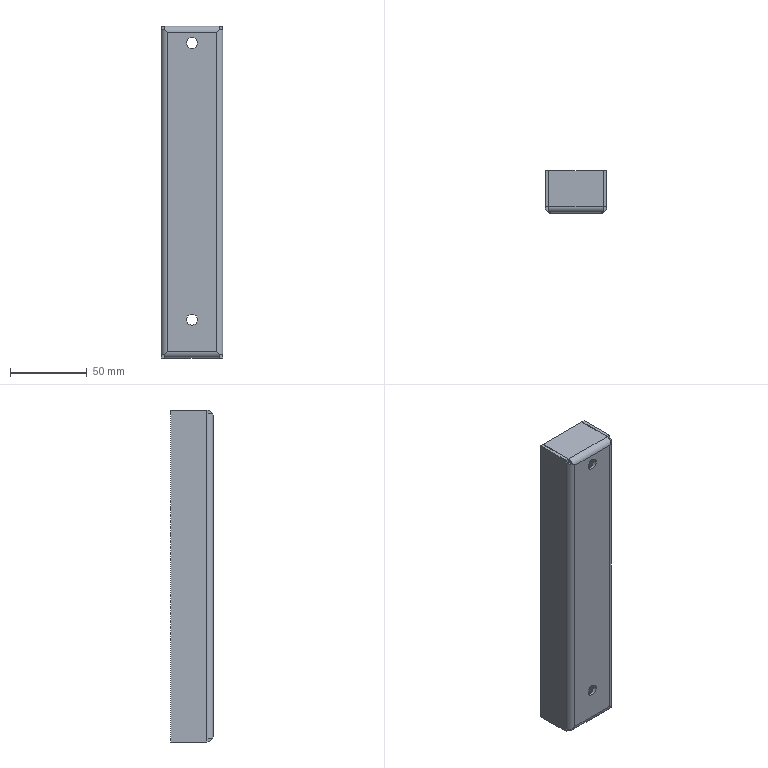Part | NX | features solid 2 | 1 solid | 50 faces | box 40 x 27.5 x 216 mm | volume 41429 mm3 | plane 38 | cylinder 12 | commonest cylinder face diameters 4 x4 7.2 x4 8 x4
STEP:
#1=CARTESIAN_POINT('',(997.,-673.5,1241.));
#2=VERTEX_POINT('',#1);
#3=CARTESIAN_POINT('',(997.,-650.,1241.));
#4=VERTEX_POINT('',#3);
#5=CARTESIAN_POINT('',(997.,-677.5,1241.));
#6=DIRECTION('',(0.,1.,0.));
#7=VECTOR('',#6,1000.);
#8=LINE('',#5,#7);
#9=EDGE_CURVE('',#2,#4,#8,.T.);
#10=ORIENTED_EDGE('',*,*,#9,.F.);
#11=CARTESIAN_POINT('',(997.,-673.5,1238.8));
#12=VERTEX_POINT('',#11);
#13=CARTESIAN_POINT('',(997.,-673.5,1025.));
#14=DIRECTION('',(0.,0.,1.));
#15=VECTOR('',#14,1000.);
#16=LINE('',#13,#15);
#17=EDGE_CURVE('',#12,#2,#16,.T.);
#18=ORIENTED_EDGE('',*,*,#17,.F.);
#19=CARTESIAN_POINT('',(997.,-673.5,1027.2));
#20=VERTEX_POINT('',#19);
#21=CARTESIAN_POINT('',(997.,-673.5,1025.));
#22=DIRECTION('',(0.,0.,1.));
#23=VECTOR('',#22,1000.);
#24=LINE('',#21,#23);
#25=EDGE_CURVE('',#20,#12,#24,.T.);
#26=ORIENTED_EDGE('',*,*,#25,.F.);
#27=CARTESIAN_POINT('',(997.,-673.5,1025.));
#28=VERTEX_POINT('',#27);
#29=CARTESIAN_POINT('',(997.,-673.5,1025.));
#30=DIRECTION('',(0.,0.,1.));
#31=VECTOR('',#30,1000.);
#32=LINE('',#29,#31);
#33=EDGE_CURVE('',#28,#20,#32,.T.);
#34=ORIENTED_EDGE('',*,*,#33,.F.);
#35=CARTESIAN_POINT('',(997.,-650.,1025.));
#36=VERTEX_POINT('',#35);
#37=CARTESIAN_POINT('',(997.,-677.5,1025.));
#38=DIRECTION('',(0.,1.,0.));
#39=VECTOR('',#38,1000.);
#40=LINE('',#37,#39);
#41=EDGE_CURVE('',#28,#36,#40,.T.);
#42=ORIENTED_EDGE('',*,*,#41,.T.);
#43=CARTESIAN_POINT('',(997.,-650.,1025.));
#44=DIRECTION('',(0.,0.,1.));
#45=VECTOR('',#44,1000.);
#46=LINE('',#43,#45);
#47=EDGE_CURVE('',#36,#4,#46,.T.);
#48=ORIENTED_EDGE('',*,*,#47,.T.);
#49=EDGE_LOOP('',(#10,#18,#26,#34,#42,#48));
#50=FACE_BOUND('',#49,.T.);
#51=CARTESIAN_POINT('',(997.,-677.5,1025.));
#52=DIRECTION('',(1.,0.,0.));
#53=DIRECTION('',(0.,0.,-1.));
#54=AXIS2_PLACEMENT_3D('',#51,#52,#53);
#55=PLANE('',#54);
#56=ADVANCED_FACE('',(#50),#55,.T.);
#57=CARTESIAN_POINT('',(995.,-673.5,1241.));
#58=VERTEX_POINT('',#57);
#59=CARTESIAN_POINT('',(995.,-650.,1241.));
#60=VERTEX_POINT('',#59);
#61=CARTESIAN_POINT('',(995.,-677.5,1241.));
#62=DIRECTION('',(0.,1.,0.));
#63=VECTOR('',#62,1000.);
#64=LINE('',#61,#63);
#65=EDGE_CURVE('',#58,#60,#64,.T.);
#66=ORIENTED_EDGE('',*,*,#65,.T.);
#67=CARTESIAN_POINT('',(995.,-650.,1025.));
#68=VERTEX_POINT('',#67);
#69=CARTESIAN_POINT('',(995.,-650.,1025.));
#70=DIRECTION('',(0.,0.,1.));
#71=VECTOR('',#70,1000.);
#72=LINE('',#69,#71);
#73=EDGE_CURVE('',#68,#60,#72,.T.);
#74=ORIENTED_EDGE('',*,*,#73,.F.);
#75=CARTESIAN_POINT('',(995.,-673.5,1025.));
#76=VERTEX_POINT('',#75);
#77=CARTESIAN_POINT('',(995.,-677.5,1025.));
#78=DIRECTION('',(0.,1.,0.));
#79=VECTOR('',#78,1000.);
#80=LINE('',#77,#79);
#81=EDGE_CURVE('',#76,#68,#80,.T.);
#82=ORIENTED_EDGE('',*,*,#81,.F.);
#83=CARTESIAN_POINT('',(995.,-673.5,1027.2));
#84=VERTEX_POINT('',#83);
#85=CARTESIAN_POINT('',(995.,-673.5,1025.));
#86=DIRECTION('',(0.,0.,1.));
#87=VECTOR('',#86,1000.);
#88=LINE('',#85,#87);
#89=EDGE_CURVE('',#76,#84,#88,.T.);
#90=ORIENTED_EDGE('',*,*,#89,.T.);
#91=CARTESIAN_POINT('',(995.,-673.5,1238.8));
#92=VERTEX_POINT('',#91);
#93=CARTESIAN_POINT('',(995.,-673.5,1025.));
#94=DIRECTION('',(0.,0.,1.));
#95=VECTOR('',#94,1000.);
#96=LINE('',#93,#95);
#97=EDGE_CURVE('',#84,#92,#96,.T.);
#98=ORIENTED_EDGE('',*,*,#97,.T.);
#99=CARTESIAN_POINT('',(995.,-673.5,1025.));
#100=DIRECTION('',(0.,0.,1.));
#101=VECTOR('',#100,1000.);
#102=LINE('',#99,#101);
#103=EDGE_CURVE('',#92,#58,#102,.T.);
#104=ORIENTED_EDGE('',*,*,#103,.T.);
#105=EDGE_LOOP('',(#66,#74,#82,#90,#98,#104));
#106=FACE_BOUND('',#105,.T.);
#107=CARTESIAN_POINT('',(995.,-677.5,1025.));
#108=DIRECTION('',(1.,0.,0.));
#109=DIRECTION('',(0.,0.,-1.));
#110=AXIS2_PLACEMENT_3D('',#107,#108,#109);
#111=PLANE('',#110);
#112=ADVANCED_FACE('',(#106),#111,.F.);
#113=CARTESIAN_POINT('',(1024.5,-673.5,1238.8));
#114=DIRECTION('',(-1.,0.,0.));
#115=VECTOR('',#114,1000.);
#116=LINE('',#113,#115);
#117=EDGE_CURVE('',#12,#92,#116,.T.);
#118=ORIENTED_EDGE('',*,*,#117,.F.);
#119=ORIENTED_EDGE('',*,*,#17,.T.);
#120=CARTESIAN_POINT('',(995.,-673.5,1241.));
#121=DIRECTION('',(1.,0.,0.));
#122=VECTOR('',#121,1000.);
#123=LINE('',#120,#122);
#124=EDGE_CURVE('',#58,#2,#123,.T.);
#125=ORIENTED_EDGE('',*,*,#124,.F.);
#126=ORIENTED_EDGE('',*,*,#103,.F.);
#127=EDGE_LOOP('',(#118,#119,#125,#126));
#128=FACE_BOUND('',#127,.T.);
#129=CARTESIAN_POINT('',(995.,-673.5,1025.));
#130=DIRECTION('',(0.,1.,0.));
#131=DIRECTION('',(1.,0.,0.));
#132=AXIS2_PLACEMENT_3D('',#129,#130,#131);
#133=PLANE('',#132);
#134=ADVANCED_FACE('',(#128),#133,.F.);
#135=CARTESIAN_POINT('',(995.,-673.5,1025.));
#136=DIRECTION('',(1.,0.,0.));
#137=VECTOR('',#136,1000.);
#138=LINE('',#135,#137);
#139=EDGE_CURVE('',#76,#28,#138,.T.);
#140=ORIENTED_EDGE('',*,*,#139,.F.);
#141=ORIENTED_EDGE('',*,*,#81,.T.);
#142=CARTESIAN_POINT('',(995.,-650.,1025.));
#143=DIRECTION('',(-1.,0.,0.));
#144=VECTOR('',#143,1000.);
#145=LINE('',#142,#144);
#146=EDGE_CURVE('',#36,#68,#145,.T.);
#147=ORIENTED_EDGE('',*,*,#146,.F.);
#148=ORIENTED_EDGE('',*,*,#41,.F.);
#149=EDGE_LOOP('',(#140,#141,#147,#148));
#150=FACE_BOUND('',#149,.T.);
#151=CARTESIAN_POINT('',(1035.,-677.5,1025.));
#152=DIRECTION('',(0.,0.,-1.));
#153=DIRECTION('',(-1.,0.,0.));
#154=AXIS2_PLACEMENT_3D('',#151,#152,#153);
#155=PLANE('',#154);
#156=ADVANCED_FACE('',(#150),#155,.T.);
#157=ORIENTED_EDGE('',*,*,#124,.T.);
#158=ORIENTED_EDGE('',*,*,#9,.T.);
#159=CARTESIAN_POINT('',(995.,-650.,1241.));
#160=DIRECTION('',(-1.,0.,0.));
#161=VECTOR('',#160,1000.);
#162=LINE('',#159,#161);
#163=EDGE_CURVE('',#4,#60,#162,.T.);
#164=ORIENTED_EDGE('',*,*,#163,.T.);
#165=ORIENTED_EDGE('',*,*,#65,.F.);
#166=EDGE_LOOP('',(#157,#158,#164,#165));
#167=FACE_BOUND('',#166,.T.);
#168=CARTESIAN_POINT('',(1031.,-673.5,1241.));
#169=DIRECTION('',(0.,0.,-1.));
#170=DIRECTION('',(-1.,0.,0.));
#171=AXIS2_PLACEMENT_3D('',#168,#169,#170);
#172=PLANE('',#171);
#173=ADVANCED_FACE('',(#167),#172,.F.);
#174=ORIENTED_EDGE('',*,*,#163,.F.);
#175=ORIENTED_EDGE('',*,*,#47,.F.);
#176=ORIENTED_EDGE('',*,*,#146,.T.);
#177=ORIENTED_EDGE('',*,*,#73,.T.);
#178=EDGE_LOOP('',(#174,#175,#176,#177));
#179=FACE_BOUND('',#178,.T.);
#180=CARTESIAN_POINT('',(995.,-650.,1025.));
#181=DIRECTION('',(0.,1.,0.));
#182=DIRECTION('',(1.,0.,0.));
#183=AXIS2_PLACEMENT_3D('',#180,#181,#182);
#184=PLANE('',#183);
#185=ADVANCED_FACE('',(#179),#184,.T.);
#186=ORIENTED_EDGE('',*,*,#33,.T.);
#187=CARTESIAN_POINT('',(1024.5,-673.5,1027.2));
#188=DIRECTION('',(-1.,0.,0.));
#189=VECTOR('',#188,1000.);
#190=LINE('',#187,#189);
#191=EDGE_CURVE('',#20,#84,#190,.T.);
#192=ORIENTED_EDGE('',*,*,#191,.T.);
#193=ORIENTED_EDGE('',*,*,#89,.F.);
#194=ORIENTED_EDGE('',*,*,#139,.T.);
#195=EDGE_LOOP('',(#186,#192,#193,#194));
#196=FACE_BOUND('',#195,.T.);
#197=CARTESIAN_POINT('',(995.,-673.5,1025.));
#198=DIRECTION('',(0.,1.,0.));
#199=DIRECTION('',(1.,0.,0.));
#200=AXIS2_PLACEMENT_3D('',#197,#198,#199);
#201=PLANE('',#200);
#202=ADVANCED_FACE('',(#196),#201,.F.);
#203=CARTESIAN_POINT('',(997.,-676.964,1238.8));
#204=VERTEX_POINT('',#203);
#205=CARTESIAN_POINT('',(999.,-673.5,1238.8));
#206=DIRECTION('',(0.,0.,-1.));
#207=DIRECTION('',(0.,1.,0.));
#208=AXIS2_PLACEMENT_3D('',#205,#206,#207);
#209=CIRCLE('',#208,4.);
#210=EDGE_CURVE('',#204,#92,#209,.T.);
#211=ORIENTED_EDGE('',*,*,#210,.F.);
#212=CARTESIAN_POINT('',(997.,322.5,1238.8));
#213=DIRECTION('',(0.,1.,0.));
#214=VECTOR('',#213,1000.);
#215=LINE('',#212,#214);
#216=EDGE_CURVE('',#204,#12,#215,.T.);
#217=ORIENTED_EDGE('',*,*,#216,.T.);
#218=ORIENTED_EDGE('',*,*,#117,.T.);
#219=EDGE_LOOP('',(#211,#217,#218));
#220=FACE_BOUND('',#219,.T.);
#221=CARTESIAN_POINT('',(997.,-1677.5,1238.8));
#222=DIRECTION('',(0.,0.,-1.));
#223=DIRECTION('',(-1.,0.,0.));
#224=AXIS2_PLACEMENT_3D('',#221,#222,#223);
#225=PLANE('',#224);
#226=ADVANCED_FACE('',(#220),#225,.F.);
#227=CARTESIAN_POINT('',(999.,-677.5,1237.));
#228=VERTEX_POINT('',#227);
#229=CARTESIAN_POINT('',(999.,-677.5,1237.));
#230=CARTESIAN_POINT('',(998.294,-677.5,1237.636));
#231=CARTESIAN_POINT('',(997.612,-677.317,1238.25));
#232=CARTESIAN_POINT('',(997.,-676.964,1238.8));
#233=(BOUNDED_CURVE()B_SPLINE_CURVE(3,(#229,#230,#231,#232),.UNSPECIFIED.,.F.,.F.)B_SPLINE_CURVE_WITH_KNOTS((4,4),(4.712,5.236),.PIECEWISE_BEZIER_KNOTS.)CURVE()GEOMETRIC_REPRESENTATION_ITEM()RATIONAL_B_SPLINE_CURVE((1.,0.9773,0.9773,1.))REPRESENTATION_ITEM(''));
#234=EDGE_CURVE('',#228,#204,#233,.T.);
#235=ORIENTED_EDGE('',*,*,#234,.F.);
#236=CARTESIAN_POINT('',(999.,-675.5,1237.));
#237=VERTEX_POINT('',#236);
#238=CARTESIAN_POINT('',(999.,-675.5,1237.));
#239=DIRECTION('',(0.,-1.,0.));
#240=VECTOR('',#239,1000.);
#241=LINE('',#238,#240);
#242=EDGE_CURVE('',#237,#228,#241,.T.);
#243=ORIENTED_EDGE('',*,*,#242,.F.);
#244=CARTESIAN_POINT('',(999.,-675.5,1237.));
#245=CARTESIAN_POINT('',(997.828,-675.5,1238.054));
#246=CARTESIAN_POINT('',(997.,-674.672,1238.8));
#247=CARTESIAN_POINT('',(997.,-673.5,1238.8));
#248=(BOUNDED_CURVE()B_SPLINE_CURVE(3,(#244,#245,#246,#247),.UNSPECIFIED.,.F.,.F.)B_SPLINE_CURVE_WITH_KNOTS((4,4),(4.712,6.283),.PIECEWISE_BEZIER_KNOTS.)CURVE()GEOMETRIC_REPRESENTATION_ITEM()RATIONAL_B_SPLINE_CURVE((1.,0.8047,0.8047,1.))REPRESENTATION_ITEM(''));
#249=EDGE_CURVE('',#237,#12,#248,.T.);
#250=ORIENTED_EDGE('',*,*,#249,.T.);
#251=ORIENTED_EDGE('',*,*,#216,.F.);
#252=EDGE_LOOP('',(#235,#243,#250,#251));
#253=FACE_BOUND('',#252,.T.);
#254=CARTESIAN_POINT('',(1742.294,-1677.5,568.035));
#255=DIRECTION('',(-0.669,0.,-0.7433));
#256=DIRECTION('',(-0.7433,0.,0.669));
#257=AXIS2_PLACEMENT_3D('',#254,#255,#256);
#258=PLANE('',#257);
#259=ADVANCED_FACE('',(#253),#258,.F.);
#260=CARTESIAN_POINT('',(997.,-676.964,1027.2));
#261=VERTEX_POINT('',#260);
#262=CARTESIAN_POINT('',(997.,322.5,1027.2));
#263=DIRECTION('',(0.,1.,0.));
#264=VECTOR('',#263,1000.);
#265=LINE('',#262,#264);
#266=EDGE_CURVE('',#261,#20,#265,.T.);
#267=ORIENTED_EDGE('',*,*,#266,.F.);
#268=CARTESIAN_POINT('',(999.,-673.5,1027.2));
#269=DIRECTION('',(0.,0.,-1.));
#270=DIRECTION('',(0.,1.,0.));
#271=AXIS2_PLACEMENT_3D('',#268,#269,#270);
#272=CIRCLE('',#271,4.);
#273=EDGE_CURVE('',#261,#84,#272,.T.);
#274=ORIENTED_EDGE('',*,*,#273,.T.);
#275=ORIENTED_EDGE('',*,*,#191,.F.);
#276=EDGE_LOOP('',(#267,#274,#275));
#277=FACE_BOUND('',#276,.T.);
#278=CARTESIAN_POINT('',(997.,-1677.5,1027.2));
#279=DIRECTION('',(0.,0.,-1.));
#280=DIRECTION('',(-1.,0.,0.));
#281=AXIS2_PLACEMENT_3D('',#278,#279,#280);
#282=PLANE('',#281);
#283=ADVANCED_FACE('',(#277),#282,.T.);
#284=CARTESIAN_POINT('',(999.,-675.5,1029.));
#285=VERTEX_POINT('',#284);
#286=CARTESIAN_POINT('',(999.,-677.5,1029.));
#287=VERTEX_POINT('',#286);
#288=CARTESIAN_POINT('',(999.,-675.5,1029.));
#289=DIRECTION('',(0.,-1.,0.));
#290=VECTOR('',#289,1000.);
#291=LINE('',#288,#290);
#292=EDGE_CURVE('',#285,#287,#291,.T.);
#293=ORIENTED_EDGE('',*,*,#292,.T.);
#294=CARTESIAN_POINT('',(999.,-677.5,1029.));
#295=CARTESIAN_POINT('',(998.294,-677.5,1028.364));
#296=CARTESIAN_POINT('',(997.612,-677.317,1027.75));
#297=CARTESIAN_POINT('',(997.,-676.964,1027.2));
#298=(BOUNDED_CURVE()B_SPLINE_CURVE(3,(#294,#295,#296,#297),.UNSPECIFIED.,.F.,.F.)B_SPLINE_CURVE_WITH_KNOTS((4,4),(1.571,2.094),.PIECEWISE_BEZIER_KNOTS.)CURVE()GEOMETRIC_REPRESENTATION_ITEM()RATIONAL_B_SPLINE_CURVE((1.,0.9773,0.9773,1.))REPRESENTATION_ITEM(''));
#299=EDGE_CURVE('',#287,#261,#298,.T.);
#300=ORIENTED_EDGE('',*,*,#299,.T.);
#301=ORIENTED_EDGE('',*,*,#266,.T.);
#302=CARTESIAN_POINT('',(999.,-675.5,1029.));
#303=CARTESIAN_POINT('',(997.828,-675.5,1027.946));
#304=CARTESIAN_POINT('',(997.,-674.672,1027.2));
#305=CARTESIAN_POINT('',(997.,-673.5,1027.2));
#306=(BOUNDED_CURVE()B_SPLINE_CURVE(3,(#302,#303,#304,#305),.UNSPECIFIED.,.F.,.F.)B_SPLINE_CURVE_WITH_KNOTS((4,4),(1.571,3.142),.PIECEWISE_BEZIER_KNOTS.)CURVE()GEOMETRIC_REPRESENTATION_ITEM()RATIONAL_B_SPLINE_CURVE((1.,0.8047,0.8047,1.))REPRESENTATION_ITEM(''));
#307=EDGE_CURVE('',#285,#20,#306,.T.);
#308=ORIENTED_EDGE('',*,*,#307,.F.);
#309=EDGE_LOOP('',(#293,#300,#301,#308));
#310=FACE_BOUND('',#309,.T.);
#311=CARTESIAN_POINT('',(1742.294,-1677.5,1697.965));
#312=DIRECTION('',(0.669,0.,-0.7433));
#313=DIRECTION('',(0.,-1.,0.));
#314=AXIS2_PLACEMENT_3D('',#311,#312,#313);
#315=PLANE('',#314);
#316=ADVANCED_FACE('',(#310),#315,.T.);
#317=ORIENTED_EDGE('',*,*,#249,.F.);
#318=CARTESIAN_POINT('',(999.,-675.5,1025.));
#319=DIRECTION('',(0.,0.,1.));
#320=VECTOR('',#319,1000.);
#321=LINE('',#318,#320);
#322=EDGE_CURVE('',#285,#237,#321,.T.);
#323=ORIENTED_EDGE('',*,*,#322,.F.);
#324=ORIENTED_EDGE('',*,*,#307,.T.);
#325=ORIENTED_EDGE('',*,*,#25,.T.);
#326=EDGE_LOOP('',(#317,#323,#324,#325));
#327=FACE_BOUND('',#326,.T.);
#328=CARTESIAN_POINT('',(999.,-673.5,1025.));
#329=DIRECTION('',(0.,0.,1.));
#330=DIRECTION('',(0.,-1.,0.));
#331=AXIS2_PLACEMENT_3D('',#328,#329,#330);
#332=CYLINDRICAL_SURFACE('',#331,2.);
#333=ADVANCED_FACE('',(#327),#332,.F.);
#334=CARTESIAN_POINT('',(999.,-677.5,1025.));
#335=DIRECTION('',(0.,0.,1.));
#336=VECTOR('',#335,1000.);
#337=LINE('',#334,#336);
#338=EDGE_CURVE('',#287,#228,#337,.T.);
#339=ORIENTED_EDGE('',*,*,#338,.T.);
#340=ORIENTED_EDGE('',*,*,#234,.T.);
#341=ORIENTED_EDGE('',*,*,#210,.T.);
#342=ORIENTED_EDGE('',*,*,#97,.F.);
#343=ORIENTED_EDGE('',*,*,#273,.F.);
#344=ORIENTED_EDGE('',*,*,#299,.F.);
#345=EDGE_LOOP('',(#339,#340,#341,#342,#343,#344));
#346=FACE_BOUND('',#345,.T.);
#347=CARTESIAN_POINT('',(999.,-673.5,1025.));
#348=DIRECTION('',(0.,0.,1.));
#349=DIRECTION('',(0.,-1.,0.));
#350=AXIS2_PLACEMENT_3D('',#347,#348,#349);
#351=CYLINDRICAL_SURFACE('',#350,4.);
#352=ADVANCED_FACE('',(#346),#351,.T.);
#353=CARTESIAN_POINT('',(997.2,-650.,1241.));
#354=VERTEX_POINT('',#353);
#355=CARTESIAN_POINT('',(997.2,-673.5,1241.));
#356=VERTEX_POINT('',#355);
#357=CARTESIAN_POINT('',(997.2,-675.778,1241.));
#358=DIRECTION('',(0.,-1.,0.));
#359=VECTOR('',#358,1000.);
#360=LINE('',#357,#359);
#361=EDGE_CURVE('',#354,#356,#360,.T.);
#362=ORIENTED_EDGE('',*,*,#361,.T.);
#363=CARTESIAN_POINT('',(1032.8,-673.5,1241.));
#364=VERTEX_POINT('',#363);
#365=CARTESIAN_POINT('',(999.,-673.5,1241.));
#366=DIRECTION('',(1.,0.,0.));
#367=VECTOR('',#366,1000.);
#368=LINE('',#365,#367);
#369=EDGE_CURVE('',#356,#364,#368,.T.);
#370=ORIENTED_EDGE('',*,*,#369,.T.);
#371=CARTESIAN_POINT('',(1032.8,-650.,1241.));
#372=VERTEX_POINT('',#371);
#373=CARTESIAN_POINT('',(1032.8,-675.778,1241.));
#374=DIRECTION('',(0.,1.,0.));
#375=VECTOR('',#374,1000.);
#376=LINE('',#373,#375);
#377=EDGE_CURVE('',#364,#372,#376,.T.);
#378=ORIENTED_EDGE('',*,*,#377,.T.);
#379=CARTESIAN_POINT('',(1031.,-650.,1241.));
#380=DIRECTION('',(-1.,0.,0.));
#381=VECTOR('',#380,1000.);
#382=LINE('',#379,#381);
#383=EDGE_CURVE('',#372,#354,#382,.T.);
#384=ORIENTED_EDGE('',*,*,#383,.T.);
#385=EDGE_LOOP('',(#362,#370,#378,#384));
#386=FACE_BOUND('',#385,.T.);
#387=CARTESIAN_POINT('',(1024.5,-552.5,1241.));
#388=DIRECTION('',(0.,0.,1.));
#389=DIRECTION('',(1.,0.,0.));
#390=AXIS2_PLACEMENT_3D('',#387,#388,#389);
#391=PLANE('',#390);
#392=ADVANCED_FACE('',(#386),#391,.T.);
#393=CARTESIAN_POINT('',(997.2,-673.5,1239.));
#394=VERTEX_POINT('',#393);
#395=CARTESIAN_POINT('',(1032.8,-673.5,1239.));
#396=VERTEX_POINT('',#395);
#397=CARTESIAN_POINT('',(999.,-673.5,1239.));
#398=DIRECTION('',(1.,0.,0.));
#399=VECTOR('',#398,1000.);
#400=LINE('',#397,#399);
#401=EDGE_CURVE('',#394,#396,#400,.T.);
#402=ORIENTED_EDGE('',*,*,#401,.F.);
#403=CARTESIAN_POINT('',(997.2,-650.,1239.));
#404=VERTEX_POINT('',#403);
#405=CARTESIAN_POINT('',(997.2,-675.778,1239.));
#406=DIRECTION('',(0.,-1.,0.));
#407=VECTOR('',#406,1000.);
#408=LINE('',#405,#407);
#409=EDGE_CURVE('',#404,#394,#408,.T.);
#410=ORIENTED_EDGE('',*,*,#409,.F.);
#411=CARTESIAN_POINT('',(1032.8,-650.,1239.));
#412=VERTEX_POINT('',#411);
#413=CARTESIAN_POINT('',(1031.,-650.,1239.));
#414=DIRECTION('',(-1.,0.,0.));
#415=VECTOR('',#414,1000.);
#416=LINE('',#413,#415);
#417=EDGE_CURVE('',#412,#404,#416,.T.);
#418=ORIENTED_EDGE('',*,*,#417,.F.);
#419=CARTESIAN_POINT('',(1032.8,-675.778,1239.));
#420=DIRECTION('',(0.,1.,0.));
#421=VECTOR('',#420,1000.);
#422=LINE('',#419,#421);
#423=EDGE_CURVE('',#396,#412,#422,.T.);
#424=ORIENTED_EDGE('',*,*,#423,.F.);
#425=EDGE_LOOP('',(#402,#410,#418,#424));
#426=FACE_BOUND('',#425,.T.);
#427=CARTESIAN_POINT('',(1024.5,-552.5,1239.));
#428=DIRECTION('',(0.,0.,1.));
#429=DIRECTION('',(1.,0.,0.));
#430=AXIS2_PLACEMENT_3D('',#427,#428,#429);
#431=PLANE('',#430);
#432=ADVANCED_FACE('',(#426),#431,.F.);
#433=ORIENTED_EDGE('',*,*,#417,.T.);
#434=CARTESIAN_POINT('',(997.2,-650.,1241.));
#435=DIRECTION('',(0.,0.,-1.));
#436=VECTOR('',#435,1000.);
#437=LINE('',#434,#436);
#438=EDGE_CURVE('',#354,#404,#437,.T.);
#439=ORIENTED_EDGE('',*,*,#438,.F.);
#440=ORIENTED_EDGE('',*,*,#383,.F.);
#441=CARTESIAN_POINT('',(1032.8,-650.,1241.));
#442=DIRECTION('',(0.,0.,-1.));
#443=VECTOR('',#442,1000.);
#444=LINE('',#441,#443);
#445=EDGE_CURVE('',#372,#412,#444,.T.);
#446=ORIENTED_EDGE('',*,*,#445,.T.);
#447=EDGE_LOOP('',(#433,#439,#440,#446));
#448=FACE_BOUND('',#447,.T.);
#449=CARTESIAN_POINT('',(1031.,-650.,1241.));
#450=DIRECTION('',(0.,-1.,0.));
#451=DIRECTION('',(0.,0.,-1.));
#452=AXIS2_PLACEMENT_3D('',#449,#450,#451);
#453=PLANE('',#452);
#454=ADVANCED_FACE('',(#448),#453,.F.);
#455=CARTESIAN_POINT('',(997.2,-676.964,1239.));
#456=VERTEX_POINT('',#455);
#457=CARTESIAN_POINT('',(997.2,-673.5,1237.));
#458=DIRECTION('',(1.,0.,0.));
#459=DIRECTION('',(0.,0.,-1.));
#460=AXIS2_PLACEMENT_3D('',#457,#458,#459);
#461=CIRCLE('',#460,4.);
#462=EDGE_CURVE('',#356,#456,#461,.T.);
#463=ORIENTED_EDGE('',*,*,#462,.F.);
#464=ORIENTED_EDGE('',*,*,#361,.F.);
#465=ORIENTED_EDGE('',*,*,#438,.T.);
#466=ORIENTED_EDGE('',*,*,#409,.T.);
#467=CARTESIAN_POINT('',(997.2,322.5,1239.));
#468=DIRECTION('',(0.,1.,0.));
#469=VECTOR('',#468,1000.);
#470=LINE('',#467,#469);
#471=EDGE_CURVE('',#456,#394,#470,.T.);
#472=ORIENTED_EDGE('',*,*,#471,.F.);
#473=EDGE_LOOP('',(#463,#464,#465,#466,#472));
#474=FACE_BOUND('',#473,.T.);
#475=CARTESIAN_POINT('',(997.2,-1677.5,1239.));
#476=DIRECTION('',(-1.,0.,0.));
#477=DIRECTION('',(0.,1.,0.));
#478=AXIS2_PLACEMENT_3D('',#475,#476,#477);
#479=PLANE('',#478);
#480=ADVANCED_FACE('',(#474),#479,.T.);
#481=ORIENTED_EDGE('',*,*,#471,.T.);
#482=CARTESIAN_POINT('',(997.2,-673.5,1239.));
#483=CARTESIAN_POINT('',(997.2,-674.672,1239.));
#484=CARTESIAN_POINT('',(997.946,-675.5,1238.172));
#485=CARTESIAN_POINT('',(999.,-675.5,1237.));
#486=(BOUNDED_CURVE()B_SPLINE_CURVE(3,(#482,#483,#484,#485),.UNSPECIFIED.,.F.,.F.)B_SPLINE_CURVE_WITH_KNOTS((4,4),(0.,1.571),.PIECEWISE_BEZIER_KNOTS.)CURVE()GEOMETRIC_REPRESENTATION_ITEM()RATIONAL_B_SPLINE_CURVE((1.,0.8047,0.8047,1.))REPRESENTATION_ITEM(''));
#487=EDGE_CURVE('',#394,#237,#486,.T.);
#488=ORIENTED_EDGE('',*,*,#487,.T.);
#489=ORIENTED_EDGE('',*,*,#242,.T.);
#490=CARTESIAN_POINT('',(997.2,-676.964,1239.));
#491=CARTESIAN_POINT('',(997.75,-677.317,1238.388));
#492=CARTESIAN_POINT('',(998.364,-677.5,1237.706));
#493=CARTESIAN_POINT('',(999.,-677.5,1237.));
#494=(BOUNDED_CURVE()B_SPLINE_CURVE(3,(#490,#491,#492,#493),.UNSPECIFIED.,.F.,.F.)B_SPLINE_CURVE_WITH_KNOTS((4,4),(1.047,1.571),.PIECEWISE_BEZIER_KNOTS.)CURVE()GEOMETRIC_REPRESENTATION_ITEM()RATIONAL_B_SPLINE_CURVE((1.,0.9773,0.9773,1.))REPRESENTATION_ITEM(''));
#495=EDGE_CURVE('',#456,#228,#494,.T.);
#496=ORIENTED_EDGE('',*,*,#495,.F.);
#497=EDGE_LOOP('',(#481,#488,#489,#496));
#498=FACE_BOUND('',#497,.T.);
#499=CARTESIAN_POINT('',(1667.965,-1677.5,493.706));
#500=DIRECTION('',(-0.7433,0.,-0.669));
#501=DIRECTION('',(-0.669,0.,0.7433));
#502=AXIS2_PLACEMENT_3D('',#499,#500,#501);
#503=PLANE('',#502);
#504=ADVANCED_FACE('',(#498),#503,.T.);
#505=CARTESIAN_POINT('',(1032.8,-676.964,1239.));
#506=VERTEX_POINT('',#505);
#507=CARTESIAN_POINT('',(1032.8,322.5,1239.));
#508=DIRECTION('',(0.,1.,0.));
#509=VECTOR('',#508,1000.);
#510=LINE('',#507,#509);
#511=EDGE_CURVE('',#506,#396,#510,.T.);
#512=ORIENTED_EDGE('',*,*,#511,.T.);
#513=ORIENTED_EDGE('',*,*,#423,.T.);
#514=ORIENTED_EDGE('',*,*,#445,.F.);
#515=ORIENTED_EDGE('',*,*,#377,.F.);
#516=CARTESIAN_POINT('',(1032.8,-673.5,1237.));
#517=DIRECTION('',(1.,0.,0.));
#518=DIRECTION('',(0.,-1.,0.));
#519=AXIS2_PLACEMENT_3D('',#516,#517,#518);
#520=CIRCLE('',#519,4.);
#521=EDGE_CURVE('',#364,#506,#520,.T.);
#522=ORIENTED_EDGE('',*,*,#521,.T.);
#523=EDGE_LOOP('',(#512,#513,#514,#515,#522));
#524=FACE_BOUND('',#523,.T.);
#525=CARTESIAN_POINT('',(1032.8,-1677.5,1239.));
#526=DIRECTION('',(-1.,0.,0.));
#527=DIRECTION('',(0.,1.,0.));
#528=AXIS2_PLACEMENT_3D('',#525,#526,#527);
#529=PLANE('',#528);
#530=ADVANCED_FACE('',(#524),#529,.F.);
#531=ORIENTED_EDGE('',*,*,#511,.F.);
#532=CARTESIAN_POINT('',(1031.,-677.5,1237.));
#533=VERTEX_POINT('',#532);
#534=CARTESIAN_POINT('',(1032.8,-676.964,1239.));
#535=CARTESIAN_POINT('',(1032.25,-677.317,1238.388));
#536=CARTESIAN_POINT('',(1031.636,-677.5,1237.706));
#537=CARTESIAN_POINT('',(1031.,-677.5,1237.));
#538=(BOUNDED_CURVE()B_SPLINE_CURVE(3,(#534,#535,#536,#537),.UNSPECIFIED.,.F.,.F.)B_SPLINE_CURVE_WITH_KNOTS((4,4),(4.189,4.712),.PIECEWISE_BEZIER_KNOTS.)CURVE()GEOMETRIC_REPRESENTATION_ITEM()RATIONAL_B_SPLINE_CURVE((1.,0.9773,0.9773,1.))REPRESENTATION_ITEM(''));
#539=EDGE_CURVE('',#506,#533,#538,.T.);
#540=ORIENTED_EDGE('',*,*,#539,.T.);
#541=CARTESIAN_POINT('',(1031.,-675.5,1237.));
#542=VERTEX_POINT('',#541);
#543=CARTESIAN_POINT('',(1031.,-675.5,1237.));
#544=DIRECTION('',(0.,-1.,0.));
#545=VECTOR('',#544,1000.);
#546=LINE('',#543,#545);
#547=EDGE_CURVE('',#542,#533,#546,.T.);
#548=ORIENTED_EDGE('',*,*,#547,.F.);
#549=CARTESIAN_POINT('',(1032.8,-673.5,1239.));
#550=CARTESIAN_POINT('',(1032.8,-674.672,1239.));
#551=CARTESIAN_POINT('',(1032.054,-675.5,1238.172));
#552=CARTESIAN_POINT('',(1031.,-675.5,1237.));
#553=(BOUNDED_CURVE()B_SPLINE_CURVE(3,(#549,#550,#551,#552),.UNSPECIFIED.,.F.,.F.)B_SPLINE_CURVE_WITH_KNOTS((4,4),(3.142,4.712),.PIECEWISE_BEZIER_KNOTS.)CURVE()GEOMETRIC_REPRESENTATION_ITEM()RATIONAL_B_SPLINE_CURVE((1.,0.8047,0.8047,1.))REPRESENTATION_ITEM(''));
#554=EDGE_CURVE('',#396,#542,#553,.T.);
#555=ORIENTED_EDGE('',*,*,#554,.F.);
#556=EDGE_LOOP('',(#531,#540,#548,#555));
#557=FACE_BOUND('',#556,.T.);
#558=CARTESIAN_POINT('',(362.035,-1677.5,493.706));
#559=DIRECTION('',(-0.7433,0.,0.669));
#560=DIRECTION('',(0.,1.,0.));
#561=AXIS2_PLACEMENT_3D('',#558,#559,#560);
#562=PLANE('',#561);
#563=ADVANCED_FACE('',(#557),#562,.F.);
#564=ORIENTED_EDGE('',*,*,#462,.T.);
#565=ORIENTED_EDGE('',*,*,#495,.T.);
#566=CARTESIAN_POINT('',(1031.,-677.5,1237.));
#567=DIRECTION('',(-1.,0.,0.));
#568=VECTOR('',#567,1000.);
#569=LINE('',#566,#568);
#570=EDGE_CURVE('',#533,#228,#569,.T.);
#571=ORIENTED_EDGE('',*,*,#570,.F.);
#572=ORIENTED_EDGE('',*,*,#539,.F.);
#573=ORIENTED_EDGE('',*,*,#521,.F.);
#574=ORIENTED_EDGE('',*,*,#369,.F.);
#575=EDGE_LOOP('',(#564,#565,#571,#572,#573,#574));
#576=FACE_BOUND('',#575,.T.);
#577=CARTESIAN_POINT('',(1031.,-673.5,1237.));
#578=DIRECTION('',(-1.,0.,0.));
#579=DIRECTION('',(0.,1.,0.));
#580=AXIS2_PLACEMENT_3D('',#577,#578,#579);
#581=CYLINDRICAL_SURFACE('',#580,4.);
#582=ADVANCED_FACE('',(#576),#581,.T.);
#583=ORIENTED_EDGE('',*,*,#487,.F.);
#584=ORIENTED_EDGE('',*,*,#401,.T.);
#585=ORIENTED_EDGE('',*,*,#554,.T.);
#586=CARTESIAN_POINT('',(1031.,-675.5,1237.));
#587=DIRECTION('',(-1.,0.,0.));
#588=VECTOR('',#587,1000.);
#589=LINE('',#586,#588);
#590=EDGE_CURVE('',#542,#237,#589,.T.);
#591=ORIENTED_EDGE('',*,*,#590,.T.);
#592=EDGE_LOOP('',(#583,#584,#585,#591));
#593=FACE_BOUND('',#592,.T.);
#594=CARTESIAN_POINT('',(1031.,-673.5,1237.));
#595=DIRECTION('',(-1.,0.,0.));
#596=DIRECTION('',(0.,1.,0.));
#597=AXIS2_PLACEMENT_3D('',#594,#595,#596);
#598=CYLINDRICAL_SURFACE('',#597,2.);
#599=ADVANCED_FACE('',(#593),#598,.F.);
#600=CARTESIAN_POINT('',(1035.,-650.,1241.));
#601=VERTEX_POINT('',#600);
#602=CARTESIAN_POINT('',(1035.,-673.5,1241.));
#603=VERTEX_POINT('',#602);
#604=CARTESIAN_POINT('',(1035.,-677.5,1241.));
#605=DIRECTION('',(0.,-1.,0.));
#606=VECTOR('',#605,1000.);
#607=LINE('',#604,#606);
#608=EDGE_CURVE('',#601,#603,#607,.T.);
#609=ORIENTED_EDGE('',*,*,#608,.T.);
#610=CARTESIAN_POINT('',(1035.,-673.5,1238.8));
#611=VERTEX_POINT('',#610);
#612=CARTESIAN_POINT('',(1035.,-673.5,1025.));
#613=DIRECTION('',(0.,0.,1.));
#614=VECTOR('',#613,1000.);
#615=LINE('',#612,#614);
#616=EDGE_CURVE('',#611,#603,#615,.T.);
#617=ORIENTED_EDGE('',*,*,#616,.F.);
#618=CARTESIAN_POINT('',(1035.,-673.5,1027.2));
#619=VERTEX_POINT('',#618);
#620=CARTESIAN_POINT('',(1035.,-673.5,1025.));
#621=DIRECTION('',(0.,0.,1.));
#622=VECTOR('',#621,1000.);
#623=LINE('',#620,#622);
#624=EDGE_CURVE('',#619,#611,#623,.T.);
#625=ORIENTED_EDGE('',*,*,#624,.F.);
#626=CARTESIAN_POINT('',(1035.,-673.5,1025.));
#627=VERTEX_POINT('',#626);
#628=CARTESIAN_POINT('',(1035.,-673.5,1025.));
#629=DIRECTION('',(0.,0.,1.));
#630=VECTOR('',#629,1000.);
#631=LINE('',#628,#630);
#632=EDGE_CURVE('',#627,#619,#631,.T.);
#633=ORIENTED_EDGE('',*,*,#632,.F.);
#634=CARTESIAN_POINT('',(1035.,-650.,1025.));
#635=VERTEX_POINT('',#634);
#636=CARTESIAN_POINT('',(1035.,-677.5,1025.));
#637=DIRECTION('',(0.,-1.,0.));
#638=VECTOR('',#637,1000.);
#639=LINE('',#636,#638);
#640=EDGE_CURVE('',#635,#627,#639,.T.);
#641=ORIENTED_EDGE('',*,*,#640,.F.);
#642=CARTESIAN_POINT('',(1035.,-650.,1025.));
#643=DIRECTION('',(0.,0.,1.));
#644=VECTOR('',#643,1000.);
#645=LINE('',#642,#644);
#646=EDGE_CURVE('',#635,#601,#645,.T.);
#647=ORIENTED_EDGE('',*,*,#646,.T.);
#648=EDGE_LOOP('',(#609,#617,#625,#633,#641,#647));
#649=FACE_BOUND('',#648,.T.);
#650=CARTESIAN_POINT('',(1035.,-677.5,1025.));
#651=DIRECTION('',(-1.,0.,0.));
#652=DIRECTION('',(0.,1.,0.));
#653=AXIS2_PLACEMENT_3D('',#650,#651,#652);
#654=PLANE('',#653);
#655=ADVANCED_FACE('',(#649),#654,.F.);
#656=CARTESIAN_POINT('',(1033.,-650.,1241.));
#657=VERTEX_POINT('',#656);
#658=CARTESIAN_POINT('',(1033.,-673.5,1241.));
#659=VERTEX_POINT('',#658);
#660=CARTESIAN_POINT('',(1033.,-677.5,1241.));
#661=DIRECTION('',(0.,-1.,0.));
#662=VECTOR('',#661,1000.);
#663=LINE('',#660,#662);
#664=EDGE_CURVE('',#657,#659,#663,.T.);
#665=ORIENTED_EDGE('',*,*,#664,.F.);
#666=CARTESIAN_POINT('',(1033.,-650.,1025.));
#667=VERTEX_POINT('',#666);
#668=CARTESIAN_POINT('',(1033.,-650.,1025.));
#669=DIRECTION('',(0.,0.,1.));
#670=VECTOR('',#669,1000.);
#671=LINE('',#668,#670);
#672=EDGE_CURVE('',#667,#657,#671,.T.);
#673=ORIENTED_EDGE('',*,*,#672,.F.);
#674=CARTESIAN_POINT('',(1033.,-673.5,1025.));
#675=VERTEX_POINT('',#674);
#676=CARTESIAN_POINT('',(1033.,-677.5,1025.));
#677=DIRECTION('',(0.,-1.,0.));
#678=VECTOR('',#677,1000.);
#679=LINE('',#676,#678);
#680=EDGE_CURVE('',#667,#675,#679,.T.);
#681=ORIENTED_EDGE('',*,*,#680,.T.);
#682=CARTESIAN_POINT('',(1033.,-673.5,1027.2));
#683=VERTEX_POINT('',#682);
#684=CARTESIAN_POINT('',(1033.,-673.5,1025.));
#685=DIRECTION('',(0.,0.,1.));
#686=VECTOR('',#685,1000.);
#687=LINE('',#684,#686);
#688=EDGE_CURVE('',#675,#683,#687,.T.);
#689=ORIENTED_EDGE('',*,*,#688,.T.);
#690=CARTESIAN_POINT('',(1033.,-673.5,1238.8));
#691=VERTEX_POINT('',#690);
#692=CARTESIAN_POINT('',(1033.,-673.5,1025.));
#693=DIRECTION('',(0.,0.,1.));
#694=VECTOR('',#693,1000.);
#695=LINE('',#692,#694);
#696=EDGE_CURVE('',#683,#691,#695,.T.);
#697=ORIENTED_EDGE('',*,*,#696,.T.);
#698=CARTESIAN_POINT('',(1033.,-673.5,1025.));
#699=DIRECTION('',(0.,0.,1.));
#700=VECTOR('',#699,1000.);
#701=LINE('',#698,#700);
#702=EDGE_CURVE('',#691,#659,#701,.T.);
#703=ORIENTED_EDGE('',*,*,#702,.T.);
#704=EDGE_LOOP('',(#665,#673,#681,#689,#697,#703));
#705=FACE_BOUND('',#704,.T.);
#706=CARTESIAN_POINT('',(1033.,-677.5,1025.));
#707=DIRECTION('',(-1.,0.,0.));
#708=DIRECTION('',(0.,1.,0.));
#709=AXIS2_PLACEMENT_3D('',#706,#707,#708);
#710=PLANE('',#709);
#711=ADVANCED_FACE('',(#705),#710,.T.);
#712=ORIENTED_EDGE('',*,*,#632,.T.);
#713=CARTESIAN_POINT('',(1024.5,-673.5,1027.2));
#714=DIRECTION('',(-1.,0.,0.));
#715=VECTOR('',#714,1000.);
#716=LINE('',#713,#715);
#717=EDGE_CURVE('',#619,#683,#716,.T.);
#718=ORIENTED_EDGE('',*,*,#717,.T.);
#719=ORIENTED_EDGE('',*,*,#688,.F.);
#720=CARTESIAN_POINT('',(1035.,-673.5,1025.));
#721=DIRECTION('',(-1.,0.,0.));
#722=VECTOR('',#721,1000.);
#723=LINE('',#720,#722);
#724=EDGE_CURVE('',#627,#675,#723,.T.);
#725=ORIENTED_EDGE('',*,*,#724,.F.);
#726=EDGE_LOOP('',(#712,#718,#719,#725));
#727=FACE_BOUND('',#726,.T.);
#728=CARTESIAN_POINT('',(1035.,-673.5,1025.));
#729=DIRECTION('',(0.,-1.,0.));
#730=DIRECTION('',(0.,0.,-1.));
#731=AXIS2_PLACEMENT_3D('',#728,#729,#730);
#732=PLANE('',#731);
#733=ADVANCED_FACE('',(#727),#732,.T.);
#734=ORIENTED_EDGE('',*,*,#640,.T.);
#735=ORIENTED_EDGE('',*,*,#724,.T.);
#736=ORIENTED_EDGE('',*,*,#680,.F.);
#737=CARTESIAN_POINT('',(1035.,-650.,1025.));
#738=DIRECTION('',(1.,0.,0.));
#739=VECTOR('',#738,1000.);
#740=LINE('',#737,#739);
#741=EDGE_CURVE('',#667,#635,#740,.T.);
#742=ORIENTED_EDGE('',*,*,#741,.T.);
#743=EDGE_LOOP('',(#734,#735,#736,#742));
#744=FACE_BOUND('',#743,.T.);
#745=CARTESIAN_POINT('',(1035.,-677.5,1025.));
#746=DIRECTION('',(0.,0.,-1.));
#747=DIRECTION('',(-1.,0.,0.));
#748=AXIS2_PLACEMENT_3D('',#745,#746,#747);
#749=PLANE('',#748);
#750=ADVANCED_FACE('',(#744),#749,.T.);
#751=ORIENTED_EDGE('',*,*,#664,.T.);
#752=CARTESIAN_POINT('',(1035.,-673.5,1241.));
#753=DIRECTION('',(-1.,0.,0.));
#754=VECTOR('',#753,1000.);
#755=LINE('',#752,#754);
#756=EDGE_CURVE('',#603,#659,#755,.T.);
#757=ORIENTED_EDGE('',*,*,#756,.F.);
#758=ORIENTED_EDGE('',*,*,#608,.F.);
#759=CARTESIAN_POINT('',(1035.,-650.,1241.));
#760=DIRECTION('',(1.,0.,0.));
#761=VECTOR('',#760,1000.);
#762=LINE('',#759,#761);
#763=EDGE_CURVE('',#657,#601,#762,.T.);
#764=ORIENTED_EDGE('',*,*,#763,.F.);
#765=EDGE_LOOP('',(#751,#757,#758,#764));
#766=FACE_BOUND('',#765,.T.);
#767=CARTESIAN_POINT('',(1031.,-673.5,1241.));
#768=DIRECTION('',(0.,0.,-1.));
#769=DIRECTION('',(-1.,0.,0.));
#770=AXIS2_PLACEMENT_3D('',#767,#768,#769);
#771=PLANE('',#770);
#772=ADVANCED_FACE('',(#766),#771,.F.);
#773=ORIENTED_EDGE('',*,*,#741,.F.);
#774=ORIENTED_EDGE('',*,*,#672,.T.);
#775=ORIENTED_EDGE('',*,*,#763,.T.);
#776=ORIENTED_EDGE('',*,*,#646,.F.);
#777=EDGE_LOOP('',(#773,#774,#775,#776));
#778=FACE_BOUND('',#777,.T.);
#779=CARTESIAN_POINT('',(1035.,-650.,1025.));
#780=DIRECTION('',(0.,-1.,0.));
#781=DIRECTION('',(0.,0.,-1.));
#782=AXIS2_PLACEMENT_3D('',#779,#780,#781);
#783=PLANE('',#782);
#784=ADVANCED_FACE('',(#778),#783,.F.);
#785=ORIENTED_EDGE('',*,*,#702,.F.);
#786=CARTESIAN_POINT('',(1024.5,-673.5,1238.8));
#787=DIRECTION('',(1.,0.,0.));
#788=VECTOR('',#787,1000.);
#789=LINE('',#786,#788);
#790=EDGE_CURVE('',#691,#611,#789,.T.);
#791=ORIENTED_EDGE('',*,*,#790,.T.);
#792=ORIENTED_EDGE('',*,*,#616,.T.);
#793=ORIENTED_EDGE('',*,*,#756,.T.);
#794=EDGE_LOOP('',(#785,#791,#792,#793));
#795=FACE_BOUND('',#794,.T.);
#796=CARTESIAN_POINT('',(1035.,-673.5,1025.));
#797=DIRECTION('',(0.,-1.,0.));
#798=DIRECTION('',(0.,0.,-1.));
#799=AXIS2_PLACEMENT_3D('',#796,#797,#798);
#800=PLANE('',#799);
#801=ADVANCED_FACE('',(#795),#800,.T.);
#802=CARTESIAN_POINT('',(1031.,-675.5,1237.));
#803=CARTESIAN_POINT('',(1032.172,-675.5,1238.054));
#804=CARTESIAN_POINT('',(1033.,-674.672,1238.8));
#805=CARTESIAN_POINT('',(1033.,-673.5,1238.8));
#806=(BOUNDED_CURVE()B_SPLINE_CURVE(3,(#802,#803,#804,#805),.UNSPECIFIED.,.F.,.F.)B_SPLINE_CURVE_WITH_KNOTS((4,4),(4.712,6.283),.PIECEWISE_BEZIER_KNOTS.)CURVE()GEOMETRIC_REPRESENTATION_ITEM()RATIONAL_B_SPLINE_CURVE((1.,0.8047,0.8047,1.))REPRESENTATION_ITEM(''));
#807=EDGE_CURVE('',#542,#691,#806,.T.);
#808=ORIENTED_EDGE('',*,*,#807,.F.);
#809=ORIENTED_EDGE('',*,*,#547,.T.);
#810=CARTESIAN_POINT('',(1033.,-676.964,1238.8));
#811=VERTEX_POINT('',#810);
#812=CARTESIAN_POINT('',(1031.,-677.5,1237.));
#813=CARTESIAN_POINT('',(1031.706,-677.5,1237.636));
#814=CARTESIAN_POINT('',(1032.388,-677.317,1238.25));
#815=CARTESIAN_POINT('',(1033.,-676.964,1238.8));
#816=(BOUNDED_CURVE()B_SPLINE_CURVE(3,(#812,#813,#814,#815),.UNSPECIFIED.,.F.,.F.)B_SPLINE_CURVE_WITH_KNOTS((4,4),(4.712,5.236),.PIECEWISE_BEZIER_KNOTS.)CURVE()GEOMETRIC_REPRESENTATION_ITEM()RATIONAL_B_SPLINE_CURVE((1.,0.9773,0.9773,1.))REPRESENTATION_ITEM(''));
#817=EDGE_CURVE('',#533,#811,#816,.T.);
#818=ORIENTED_EDGE('',*,*,#817,.T.);
#819=CARTESIAN_POINT('',(1033.,322.5,1238.8));
#820=DIRECTION('',(0.,1.,0.));
#821=VECTOR('',#820,1000.);
#822=LINE('',#819,#821);
#823=EDGE_CURVE('',#811,#691,#822,.T.);
#824=ORIENTED_EDGE('',*,*,#823,.T.);
#825=EDGE_LOOP('',(#808,#809,#818,#824));
#826=FACE_BOUND('',#825,.T.);
#827=CARTESIAN_POINT('',(287.706,-1677.5,568.035));
#828=DIRECTION('',(-0.669,0.,0.7433));
#829=DIRECTION('',(0.,1.,0.));
#830=AXIS2_PLACEMENT_3D('',#827,#828,#829);
#831=PLANE('',#830);
#832=ADVANCED_FACE('',(#826),#831,.T.);
#833=ORIENTED_EDGE('',*,*,#823,.F.);
#834=CARTESIAN_POINT('',(1031.,-673.5,1238.8));
#835=DIRECTION('',(0.,0.,1.));
#836=DIRECTION('',(0.,-1.,0.));
#837=AXIS2_PLACEMENT_3D('',#834,#835,#836);
#838=CIRCLE('',#837,4.);
#839=EDGE_CURVE('',#811,#611,#838,.T.);
#840=ORIENTED_EDGE('',*,*,#839,.T.);
#841=ORIENTED_EDGE('',*,*,#790,.F.);
#842=EDGE_LOOP('',(#833,#840,#841));
#843=FACE_BOUND('',#842,.T.);
#844=CARTESIAN_POINT('',(1033.,-1677.5,1238.8));
#845=DIRECTION('',(0.,0.,1.));
#846=DIRECTION('',(1.,0.,0.));
#847=AXIS2_PLACEMENT_3D('',#844,#845,#846);
#848=PLANE('',#847);
#849=ADVANCED_FACE('',(#843),#848,.T.);
#850=CARTESIAN_POINT('',(1033.,-676.964,1027.2));
#851=VERTEX_POINT('',#850);
#852=CARTESIAN_POINT('',(1031.,-673.5,1027.2));
#853=DIRECTION('',(0.,0.,1.));
#854=DIRECTION('',(0.,-1.,0.));
#855=AXIS2_PLACEMENT_3D('',#852,#853,#854);
#856=CIRCLE('',#855,4.);
#857=EDGE_CURVE('',#851,#619,#856,.T.);
#858=ORIENTED_EDGE('',*,*,#857,.F.);
#859=CARTESIAN_POINT('',(1033.,322.5,1027.2));
#860=DIRECTION('',(0.,1.,0.));
#861=VECTOR('',#860,1000.);
#862=LINE('',#859,#861);
#863=EDGE_CURVE('',#851,#683,#862,.T.);
#864=ORIENTED_EDGE('',*,*,#863,.T.);
#865=ORIENTED_EDGE('',*,*,#717,.F.);
#866=EDGE_LOOP('',(#858,#864,#865));
#867=FACE_BOUND('',#866,.T.);
#868=CARTESIAN_POINT('',(1033.,-1677.5,1027.2));
#869=DIRECTION('',(0.,0.,1.));
#870=DIRECTION('',(1.,0.,0.));
#871=AXIS2_PLACEMENT_3D('',#868,#869,#870);
#872=PLANE('',#871);
#873=ADVANCED_FACE('',(#867),#872,.F.);
#874=CARTESIAN_POINT('',(1031.,-675.5,1029.));
#875=VERTEX_POINT('',#874);
#876=CARTESIAN_POINT('',(1031.,-677.5,1029.));
#877=VERTEX_POINT('',#876);
#878=CARTESIAN_POINT('',(1031.,-675.5,1029.));
#879=DIRECTION('',(0.,-1.,0.));
#880=VECTOR('',#879,1000.);
#881=LINE('',#878,#880);
#882=EDGE_CURVE('',#875,#877,#881,.T.);
#883=ORIENTED_EDGE('',*,*,#882,.F.);
#884=CARTESIAN_POINT('',(1031.,-675.5,1029.));
#885=CARTESIAN_POINT('',(1032.172,-675.5,1027.946));
#886=CARTESIAN_POINT('',(1033.,-674.672,1027.2));
#887=CARTESIAN_POINT('',(1033.,-673.5,1027.2));
#888=(BOUNDED_CURVE()B_SPLINE_CURVE(3,(#884,#885,#886,#887),.UNSPECIFIED.,.F.,.F.)B_SPLINE_CURVE_WITH_KNOTS((4,4),(1.571,3.142),.PIECEWISE_BEZIER_KNOTS.)CURVE()GEOMETRIC_REPRESENTATION_ITEM()RATIONAL_B_SPLINE_CURVE((1.,0.8047,0.8047,1.))REPRESENTATION_ITEM(''));
#889=EDGE_CURVE('',#875,#683,#888,.T.);
#890=ORIENTED_EDGE('',*,*,#889,.T.);
#891=ORIENTED_EDGE('',*,*,#863,.F.);
#892=CARTESIAN_POINT('',(1031.,-677.5,1029.));
#893=CARTESIAN_POINT('',(1031.706,-677.5,1028.364));
#894=CARTESIAN_POINT('',(1032.388,-677.317,1027.75));
#895=CARTESIAN_POINT('',(1033.,-676.964,1027.2));
#896=(BOUNDED_CURVE()B_SPLINE_CURVE(3,(#892,#893,#894,#895),.UNSPECIFIED.,.F.,.F.)B_SPLINE_CURVE_WITH_KNOTS((4,4),(1.571,2.094),.PIECEWISE_BEZIER_KNOTS.)CURVE()GEOMETRIC_REPRESENTATION_ITEM()RATIONAL_B_SPLINE_CURVE((1.,0.9773,0.9773,1.))REPRESENTATION_ITEM(''));
#897=EDGE_CURVE('',#877,#851,#896,.T.);
#898=ORIENTED_EDGE('',*,*,#897,.F.);
#899=EDGE_LOOP('',(#883,#890,#891,#898));
#900=FACE_BOUND('',#899,.T.);
#901=CARTESIAN_POINT('',(287.706,-1677.5,1697.965));
#902=DIRECTION('',(0.669,0.,0.7433));
#903=DIRECTION('',(0.,-1.,0.));
#904=AXIS2_PLACEMENT_3D('',#901,#902,#903);
#905=PLANE('',#904);
#906=ADVANCED_FACE('',(#900),#905,.F.);
#907=ORIENTED_EDGE('',*,*,#817,.F.);
#908=CARTESIAN_POINT('',(1031.,-677.5,1025.));
#909=DIRECTION('',(0.,0.,1.));
#910=VECTOR('',#909,1000.);
#911=LINE('',#908,#910);
#912=EDGE_CURVE('',#877,#533,#911,.T.);
#913=ORIENTED_EDGE('',*,*,#912,.F.);
#914=ORIENTED_EDGE('',*,*,#897,.T.);
#915=ORIENTED_EDGE('',*,*,#857,.T.);
#916=ORIENTED_EDGE('',*,*,#624,.T.);
#917=ORIENTED_EDGE('',*,*,#839,.F.);
#918=EDGE_LOOP('',(#907,#913,#914,#915,#916,#917));
#919=FACE_BOUND('',#918,.T.);
#920=CARTESIAN_POINT('',(1031.,-673.5,1025.));
#921=DIRECTION('',(0.,0.,1.));
#922=DIRECTION('',(0.,-1.,0.));
#923=AXIS2_PLACEMENT_3D('',#920,#921,#922);
#924=CYLINDRICAL_SURFACE('',#923,4.);
#925=ADVANCED_FACE('',(#919),#924,.T.);
#926=CARTESIAN_POINT('',(1031.,-675.5,1025.));
#927=DIRECTION('',(0.,0.,1.));
#928=VECTOR('',#927,1000.);
#929=LINE('',#926,#928);
#930=EDGE_CURVE('',#875,#542,#929,.T.);
#931=ORIENTED_EDGE('',*,*,#930,.T.);
#932=ORIENTED_EDGE('',*,*,#807,.T.);
#933=ORIENTED_EDGE('',*,*,#696,.F.);
#934=ORIENTED_EDGE('',*,*,#889,.F.);
#935=EDGE_LOOP('',(#931,#932,#933,#934));
#936=FACE_BOUND('',#935,.T.);
#937=CARTESIAN_POINT('',(1031.,-673.5,1025.));
#938=DIRECTION('',(0.,0.,1.));
#939=DIRECTION('',(0.,-1.,0.));
#940=AXIS2_PLACEMENT_3D('',#937,#938,#939);
#941=CYLINDRICAL_SURFACE('',#940,2.);
#942=ADVANCED_FACE('',(#936),#941,.F.);
#943=CARTESIAN_POINT('',(1032.8,-650.,1025.));
#944=VERTEX_POINT('',#943);
#945=CARTESIAN_POINT('',(1032.8,-673.5,1025.));
#946=VERTEX_POINT('',#945);
#947=CARTESIAN_POINT('',(1032.8,-675.778,1025.));
#948=DIRECTION('',(0.,-1.,0.));
#949=VECTOR('',#948,1000.);
#950=LINE('',#947,#949);
#951=EDGE_CURVE('',#944,#946,#950,.T.);
#952=ORIENTED_EDGE('',*,*,#951,.T.);
#953=CARTESIAN_POINT('',(997.2,-673.5,1025.));
#954=VERTEX_POINT('',#953);
#955=CARTESIAN_POINT('',(1031.,-673.5,1025.));
#956=DIRECTION('',(-1.,0.,0.));
#957=VECTOR('',#956,1000.);
#958=LINE('',#955,#957);
#959=EDGE_CURVE('',#946,#954,#958,.T.);
#960=ORIENTED_EDGE('',*,*,#959,.T.);
#961=CARTESIAN_POINT('',(997.2,-650.,1025.));
#962=VERTEX_POINT('',#961);
#963=CARTESIAN_POINT('',(997.2,-675.778,1025.));
#964=DIRECTION('',(0.,1.,0.));
#965=VECTOR('',#964,1000.);
#966=LINE('',#963,#965);
#967=EDGE_CURVE('',#954,#962,#966,.T.);
#968=ORIENTED_EDGE('',*,*,#967,.T.);
#969=CARTESIAN_POINT('',(999.,-650.,1025.));
#970=DIRECTION('',(1.,0.,0.));
#971=VECTOR('',#970,1000.);
#972=LINE('',#969,#971);
#973=EDGE_CURVE('',#962,#944,#972,.T.);
#974=ORIENTED_EDGE('',*,*,#973,.T.);
#975=EDGE_LOOP('',(#952,#960,#968,#974));
#976=FACE_BOUND('',#975,.T.);
#977=CARTESIAN_POINT('',(1024.5,-552.5,1025.));
#978=DIRECTION('',(0.,0.,-1.));
#979=DIRECTION('',(-1.,0.,0.));
#980=AXIS2_PLACEMENT_3D('',#977,#978,#979);
#981=PLANE('',#980);
#982=ADVANCED_FACE('',(#976),#981,.T.);
#983=CARTESIAN_POINT('',(1032.8,-673.5,1027.));
#984=VERTEX_POINT('',#983);
#985=CARTESIAN_POINT('',(997.2,-673.5,1027.));
#986=VERTEX_POINT('',#985);
#987=CARTESIAN_POINT('',(1031.,-673.5,1027.));
#988=DIRECTION('',(-1.,0.,0.));
#989=VECTOR('',#988,1000.);
#990=LINE('',#987,#989);
#991=EDGE_CURVE('',#984,#986,#990,.T.);
#992=ORIENTED_EDGE('',*,*,#991,.F.);
#993=CARTESIAN_POINT('',(1032.8,-650.,1027.));
#994=VERTEX_POINT('',#993);
#995=CARTESIAN_POINT('',(1032.8,-675.778,1027.));
#996=DIRECTION('',(0.,-1.,0.));
#997=VECTOR('',#996,1000.);
#998=LINE('',#995,#997);
#999=EDGE_CURVE('',#994,#984,#998,.T.);
#1000=ORIENTED_EDGE('',*,*,#999,.F.);
#1001=CARTESIAN_POINT('',(997.2,-650.,1027.));
#1002=VERTEX_POINT('',#1001);
#1003=CARTESIAN_POINT('',(999.,-650.,1027.));
#1004=DIRECTION('',(1.,0.,0.));
#1005=VECTOR('',#1004,1000.);
#1006=LINE('',#1003,#1005);
#1007=EDGE_CURVE('',#1002,#994,#1006,.T.);
#1008=ORIENTED_EDGE('',*,*,#1007,.F.);
#1009=CARTESIAN_POINT('',(997.2,-675.778,1027.));
#1010=DIRECTION('',(0.,1.,0.));
#1011=VECTOR('',#1010,1000.);
#1012=LINE('',#1009,#1011);
#1013=EDGE_CURVE('',#986,#1002,#1012,.T.);
#1014=ORIENTED_EDGE('',*,*,#1013,.F.);
#1015=EDGE_LOOP('',(#992,#1000,#1008,#1014));
#1016=FACE_BOUND('',#1015,.T.);
#1017=CARTESIAN_POINT('',(1024.5,-552.5,1027.));
#1018=DIRECTION('',(0.,0.,-1.));
#1019=DIRECTION('',(-1.,0.,0.));
#1020=AXIS2_PLACEMENT_3D('',#1017,#1018,#1019);
#1021=PLANE('',#1020);
#1022=ADVANCED_FACE('',(#1016),#1021,.F.);
#1023=ORIENTED_EDGE('',*,*,#1007,.T.);
#1024=CARTESIAN_POINT('',(1032.8,-650.,1025.));
#1025=DIRECTION('',(0.,0.,1.));
#1026=VECTOR('',#1025,1000.);
#1027=LINE('',#1024,#1026);
#1028=EDGE_CURVE('',#944,#994,#1027,.T.);
#1029=ORIENTED_EDGE('',*,*,#1028,.F.);
#1030=ORIENTED_EDGE('',*,*,#973,.F.);
#1031=CARTESIAN_POINT('',(997.2,-650.,1025.));
#1032=DIRECTION('',(0.,0.,1.));
#1033=VECTOR('',#1032,1000.);
#1034=LINE('',#1031,#1033);
#1035=EDGE_CURVE('',#962,#1002,#1034,.T.);
#1036=ORIENTED_EDGE('',*,*,#1035,.T.);
#1037=EDGE_LOOP('',(#1023,#1029,#1030,#1036));
#1038=FACE_BOUND('',#1037,.T.);
#1039=CARTESIAN_POINT('',(999.,-650.,1025.));
#1040=DIRECTION('',(0.,-1.,0.));
#1041=DIRECTION('',(0.,0.,-1.));
#1042=AXIS2_PLACEMENT_3D('',#1039,#1040,#1041);
#1043=PLANE('',#1042);
#1044=ADVANCED_FACE('',(#1038),#1043,.F.);
#1045=CARTESIAN_POINT('',(1032.8,-676.964,1027.));
#1046=VERTEX_POINT('',#1045);
#1047=CARTESIAN_POINT('',(1032.8,-673.5,1029.));
#1048=DIRECTION('',(-1.,0.,0.));
#1049=DIRECTION('',(0.,1.,0.));
#1050=AXIS2_PLACEMENT_3D('',#1047,#1048,#1049);
#1051=CIRCLE('',#1050,4.);
#1052=EDGE_CURVE('',#946,#1046,#1051,.T.);
#1053=ORIENTED_EDGE('',*,*,#1052,.F.);
#1054=ORIENTED_EDGE('',*,*,#951,.F.);
#1055=ORIENTED_EDGE('',*,*,#1028,.T.);
#1056=ORIENTED_EDGE('',*,*,#999,.T.);
#1057=CARTESIAN_POINT('',(1032.8,322.5,1027.));
#1058=DIRECTION('',(0.,1.,0.));
#1059=VECTOR('',#1058,1000.);
#1060=LINE('',#1057,#1059);
#1061=EDGE_CURVE('',#1046,#984,#1060,.T.);
#1062=ORIENTED_EDGE('',*,*,#1061,.F.);
#1063=EDGE_LOOP('',(#1053,#1054,#1055,#1056,#1062));
#1064=FACE_BOUND('',#1063,.T.);
#1065=CARTESIAN_POINT('',(1032.8,-1677.5,1027.));
#1066=DIRECTION('',(1.,0.,0.));
#1067=DIRECTION('',(0.,0.,-1.));
#1068=AXIS2_PLACEMENT_3D('',#1065,#1066,#1067);
#1069=PLANE('',#1068);
#1070=ADVANCED_FACE('',(#1064),#1069,.T.);
#1071=ORIENTED_EDGE('',*,*,#1061,.T.);
#1072=CARTESIAN_POINT('',(1032.8,-673.5,1027.));
#1073=CARTESIAN_POINT('',(1032.8,-674.672,1027.));
#1074=CARTESIAN_POINT('',(1032.054,-675.5,1027.828));
#1075=CARTESIAN_POINT('',(1031.,-675.5,1029.));
#1076=(BOUNDED_CURVE()B_SPLINE_CURVE(3,(#1072,#1073,#1074,#1075),.UNSPECIFIED.,.F.,.F.)B_SPLINE_CURVE_WITH_KNOTS((4,4),(0.,1.571),.PIECEWISE_BEZIER_KNOTS.)CURVE()GEOMETRIC_REPRESENTATION_ITEM()RATIONAL_B_SPLINE_CURVE((1.,0.8047,0.8047,1.))REPRESENTATION_ITEM(''));
#1077=EDGE_CURVE('',#984,#875,#1076,.T.);
#1078=ORIENTED_EDGE('',*,*,#1077,.T.);
#1079=ORIENTED_EDGE('',*,*,#882,.T.);
#1080=CARTESIAN_POINT('',(1032.8,-676.964,1027.));
#1081=CARTESIAN_POINT('',(1032.25,-677.317,1027.612));
#1082=CARTESIAN_POINT('',(1031.636,-677.5,1028.294));
#1083=CARTESIAN_POINT('',(1031.,-677.5,1029.));
#1084=(BOUNDED_CURVE()B_SPLINE_CURVE(3,(#1080,#1081,#1082,#1083),.UNSPECIFIED.,.F.,.F.)B_SPLINE_CURVE_WITH_KNOTS((4,4),(1.047,1.571),.PIECEWISE_BEZIER_KNOTS.)CURVE()GEOMETRIC_REPRESENTATION_ITEM()RATIONAL_B_SPLINE_CURVE((1.,0.9773,0.9773,1.))REPRESENTATION_ITEM(''));
#1085=EDGE_CURVE('',#1046,#877,#1084,.T.);
#1086=ORIENTED_EDGE('',*,*,#1085,.F.);
#1087=EDGE_LOOP('',(#1071,#1078,#1079,#1086));
#1088=FACE_BOUND('',#1087,.T.);
#1089=CARTESIAN_POINT('',(362.035,-1677.5,1772.294));
#1090=DIRECTION('',(0.7433,0.,0.669));
#1091=DIRECTION('',(0.,-1.,0.));
#1092=AXIS2_PLACEMENT_3D('',#1089,#1090,#1091);
#1093=PLANE('',#1092);
#1094=ADVANCED_FACE('',(#1088),#1093,.T.);
#1095=CARTESIAN_POINT('',(997.2,-676.964,1027.));
#1096=VERTEX_POINT('',#1095);
#1097=CARTESIAN_POINT('',(997.2,322.5,1027.));
#1098=DIRECTION('',(0.,1.,0.));
#1099=VECTOR('',#1098,1000.);
#1100=LINE('',#1097,#1099);
#1101=EDGE_CURVE('',#1096,#986,#1100,.T.);
#1102=ORIENTED_EDGE('',*,*,#1101,.T.);
#1103=ORIENTED_EDGE('',*,*,#1013,.T.);
#1104=ORIENTED_EDGE('',*,*,#1035,.F.);
#1105=ORIENTED_EDGE('',*,*,#967,.F.);
#1106=CARTESIAN_POINT('',(997.2,-673.5,1029.));
#1107=DIRECTION('',(-1.,0.,0.));
#1108=DIRECTION('',(0.,1.,0.));
#1109=AXIS2_PLACEMENT_3D('',#1106,#1107,#1108);
#1110=CIRCLE('',#1109,4.);
#1111=EDGE_CURVE('',#954,#1096,#1110,.T.);
#1112=ORIENTED_EDGE('',*,*,#1111,.T.);
#1113=EDGE_LOOP('',(#1102,#1103,#1104,#1105,#1112));
#1114=FACE_BOUND('',#1113,.T.);
#1115=CARTESIAN_POINT('',(997.2,-1677.5,1027.));
#1116=DIRECTION('',(1.,0.,0.));
#1117=DIRECTION('',(0.,0.,-1.));
#1118=AXIS2_PLACEMENT_3D('',#1115,#1116,#1117);
#1119=PLANE('',#1118);
#1120=ADVANCED_FACE('',(#1114),#1119,.F.);
#1121=ORIENTED_EDGE('',*,*,#1101,.F.);
#1122=CARTESIAN_POINT('',(997.2,-676.964,1027.));
#1123=CARTESIAN_POINT('',(997.75,-677.317,1027.612));
#1124=CARTESIAN_POINT('',(998.364,-677.5,1028.294));
#1125=CARTESIAN_POINT('',(999.,-677.5,1029.));
#1126=(BOUNDED_CURVE()B_SPLINE_CURVE(3,(#1122,#1123,#1124,#1125),.UNSPECIFIED.,.F.,.F.)B_SPLINE_CURVE_WITH_KNOTS((4,4),(4.189,4.712),.PIECEWISE_BEZIER_KNOTS.)CURVE()GEOMETRIC_REPRESENTATION_ITEM()RATIONAL_B_SPLINE_CURVE((1.,0.9773,0.9773,1.))REPRESENTATION_ITEM(''));
#1127=EDGE_CURVE('',#1096,#287,#1126,.T.);
#1128=ORIENTED_EDGE('',*,*,#1127,.T.);
#1129=ORIENTED_EDGE('',*,*,#292,.F.);
#1130=CARTESIAN_POINT('',(997.2,-673.5,1027.));
#1131=CARTESIAN_POINT('',(997.2,-674.672,1027.));
#1132=CARTESIAN_POINT('',(997.946,-675.5,1027.828));
#1133=CARTESIAN_POINT('',(999.,-675.5,1029.));
#1134=(BOUNDED_CURVE()B_SPLINE_CURVE(3,(#1130,#1131,#1132,#1133),.UNSPECIFIED.,.F.,.F.)B_SPLINE_CURVE_WITH_KNOTS((4,4),(3.142,4.712),.PIECEWISE_BEZIER_KNOTS.)CURVE()GEOMETRIC_REPRESENTATION_ITEM()RATIONAL_B_SPLINE_CURVE((1.,0.8047,0.8047,1.))REPRESENTATION_ITEM(''));
#1135=EDGE_CURVE('',#986,#285,#1134,.T.);
#1136=ORIENTED_EDGE('',*,*,#1135,.F.);
#1137=EDGE_LOOP('',(#1121,#1128,#1129,#1136));
#1138=FACE_BOUND('',#1137,.T.);
#1139=CARTESIAN_POINT('',(1667.965,-1677.5,1772.294));
#1140=DIRECTION('',(0.7433,0.,-0.669));
#1141=DIRECTION('',(0.,-1.,0.));
#1142=AXIS2_PLACEMENT_3D('',#1139,#1140,#1141);
#1143=PLANE('',#1142);
#1144=ADVANCED_FACE('',(#1138),#1143,.F.);
#1145=ORIENTED_EDGE('',*,*,#1052,.T.);
#1146=ORIENTED_EDGE('',*,*,#1085,.T.);
#1147=CARTESIAN_POINT('',(999.,-677.5,1029.));
#1148=DIRECTION('',(1.,0.,0.));
#1149=VECTOR('',#1148,1000.);
#1150=LINE('',#1147,#1149);
#1151=EDGE_CURVE('',#287,#877,#1150,.T.);
#1152=ORIENTED_EDGE('',*,*,#1151,.F.);
#1153=ORIENTED_EDGE('',*,*,#1127,.F.);
#1154=ORIENTED_EDGE('',*,*,#1111,.F.);
#1155=ORIENTED_EDGE('',*,*,#959,.F.);
#1156=EDGE_LOOP('',(#1145,#1146,#1152,#1153,#1154,#1155));
#1157=FACE_BOUND('',#1156,.T.);
#1158=CARTESIAN_POINT('',(999.,-673.5,1029.));
#1159=DIRECTION('',(1.,0.,0.));
#1160=DIRECTION('',(0.,1.,0.));
#1161=AXIS2_PLACEMENT_3D('',#1158,#1159,#1160);
#1162=CYLINDRICAL_SURFACE('',#1161,4.);
#1163=ADVANCED_FACE('',(#1157),#1162,.T.);
#1164=ORIENTED_EDGE('',*,*,#1077,.F.);
#1165=ORIENTED_EDGE('',*,*,#991,.T.);
#1166=ORIENTED_EDGE('',*,*,#1135,.T.);
#1167=CARTESIAN_POINT('',(999.,-675.5,1029.));
#1168=DIRECTION('',(1.,0.,0.));
#1169=VECTOR('',#1168,1000.);
#1170=LINE('',#1167,#1169);
#1171=EDGE_CURVE('',#285,#875,#1170,.T.);
#1172=ORIENTED_EDGE('',*,*,#1171,.T.);
#1173=EDGE_LOOP('',(#1164,#1165,#1166,#1172));
#1174=FACE_BOUND('',#1173,.T.);
#1175=CARTESIAN_POINT('',(999.,-673.5,1029.));
#1176=DIRECTION('',(1.,0.,0.));
#1177=DIRECTION('',(0.,1.,0.));
#1178=AXIS2_PLACEMENT_3D('',#1175,#1176,#1177);
#1179=CYLINDRICAL_SURFACE('',#1178,2.);
#1180=ADVANCED_FACE('',(#1174),#1179,.F.);
#1181=CARTESIAN_POINT('',(1011.4,-677.5,1050.));
#1182=VERTEX_POINT('',#1181);
#1183=CARTESIAN_POINT('',(1011.4,-675.5,1050.));
#1184=VERTEX_POINT('',#1183);
#1185=CARTESIAN_POINT('',(1011.4,-456.113,1050.));
#1186=DIRECTION('',(0.,-1.,0.));
#1187=VECTOR('',#1186,1000.);
#1188=LINE('',#1185,#1187);
#1189=EDGE_CURVE('',#1182,#1184,#1188,.F.);
#1190=ORIENTED_EDGE('',*,*,#1189,.T.);
#1191=CARTESIAN_POINT('',(1018.6,-675.5,1050.));
#1192=VERTEX_POINT('',#1191);
#1193=CARTESIAN_POINT('',(1015.,-675.5,1050.));
#1194=DIRECTION('',(0.,1.,0.));
#1195=DIRECTION('',(-1.,0.,0.));
#1196=AXIS2_PLACEMENT_3D('',#1193,#1194,#1195);
#1197=CIRCLE('',#1196,3.6);
#1198=EDGE_CURVE('',#1184,#1192,#1197,.T.);
#1199=ORIENTED_EDGE('',*,*,#1198,.T.);
#1200=CARTESIAN_POINT('',(1018.6,-677.5,1050.));
#1201=VERTEX_POINT('',#1200);
#1202=CARTESIAN_POINT('',(1018.6,-456.113,1050.));
#1203=DIRECTION('',(0.,-1.,0.));
#1204=VECTOR('',#1203,1000.);
#1205=LINE('',#1202,#1204);
#1206=EDGE_CURVE('',#1192,#1201,#1205,.T.);
#1207=ORIENTED_EDGE('',*,*,#1206,.T.);
#1208=CARTESIAN_POINT('',(1015.,-677.5,1050.));
#1209=DIRECTION('',(0.,-1.,0.));
#1210=DIRECTION('',(0.,0.,1.));
#1211=AXIS2_PLACEMENT_3D('',#1208,#1209,#1210);
#1212=CIRCLE('',#1211,3.6);
#1213=EDGE_CURVE('',#1201,#1182,#1212,.T.);
#1214=ORIENTED_EDGE('',*,*,#1213,.T.);
#1215=EDGE_LOOP('',(#1190,#1199,#1207,#1214));
#1216=FACE_BOUND('',#1215,.T.);
#1217=CARTESIAN_POINT('',(1015.,-456.113,1050.));
#1218=DIRECTION('',(0.,-1.,0.));
#1219=DIRECTION('',(1.,0.,0.));
#1220=AXIS2_PLACEMENT_3D('',#1217,#1218,#1219);
#1221=CYLINDRICAL_SURFACE('',#1220,3.6);
#1222=ADVANCED_FACE('',(#1216),#1221,.F.);
#1223=CARTESIAN_POINT('',(1011.4,-677.5,1230.));
#1224=VERTEX_POINT('',#1223);
#1225=CARTESIAN_POINT('',(1011.4,-675.5,1230.));
#1226=VERTEX_POINT('',#1225);
#1227=CARTESIAN_POINT('',(1011.4,-456.113,1230.));
#1228=DIRECTION('',(0.,-1.,0.));
#1229=VECTOR('',#1228,1000.);
#1230=LINE('',#1227,#1229);
#1231=EDGE_CURVE('',#1224,#1226,#1230,.F.);
#1232=ORIENTED_EDGE('',*,*,#1231,.T.);
#1233=CARTESIAN_POINT('',(1018.6,-675.5,1230.));
#1234=VERTEX_POINT('',#1233);
#1235=CARTESIAN_POINT('',(1015.,-675.5,1230.));
#1236=DIRECTION('',(0.,1.,0.));
#1237=DIRECTION('',(-1.,0.,0.));
#1238=AXIS2_PLACEMENT_3D('',#1235,#1236,#1237);
#1239=CIRCLE('',#1238,3.6);
#1240=EDGE_CURVE('',#1226,#1234,#1239,.T.);
#1241=ORIENTED_EDGE('',*,*,#1240,.T.);
#1242=CARTESIAN_POINT('',(1018.6,-677.5,1230.));
#1243=VERTEX_POINT('',#1242);
#1244=CARTESIAN_POINT('',(1018.6,-456.113,1230.));
#1245=DIRECTION('',(0.,-1.,0.));
#1246=VECTOR('',#1245,1000.);
#1247=LINE('',#1244,#1246);
#1248=EDGE_CURVE('',#1234,#1243,#1247,.T.);
#1249=ORIENTED_EDGE('',*,*,#1248,.T.);
#1250=CARTESIAN_POINT('',(1015.,-677.5,1230.));
#1251=DIRECTION('',(0.,-1.,0.));
#1252=DIRECTION('',(0.,0.,1.));
#1253=AXIS2_PLACEMENT_3D('',#1250,#1251,#1252);
#1254=CIRCLE('',#1253,3.6);
#1255=EDGE_CURVE('',#1243,#1224,#1254,.T.);
#1256=ORIENTED_EDGE('',*,*,#1255,.T.);
#1257=EDGE_LOOP('',(#1232,#1241,#1249,#1256));
#1258=FACE_BOUND('',#1257,.T.);
#1259=CARTESIAN_POINT('',(1015.,-456.113,1230.));
#1260=DIRECTION('',(0.,-1.,0.));
#1261=DIRECTION('',(1.,0.,0.));
#1262=AXIS2_PLACEMENT_3D('',#1259,#1260,#1261);
#1263=CYLINDRICAL_SURFACE('',#1262,3.6);
#1264=ADVANCED_FACE('',(#1258),#1263,.F.);
#1265=CARTESIAN_POINT('',(1015.,-675.5,1230.));
#1266=DIRECTION('',(0.,1.,0.));
#1267=DIRECTION('',(-1.,0.,0.));
#1268=AXIS2_PLACEMENT_3D('',#1265,#1266,#1267);
#1269=CIRCLE('',#1268,3.6);
#1270=EDGE_CURVE('',#1234,#1226,#1269,.T.);
#1271=ORIENTED_EDGE('',*,*,#1270,.F.);
#1272=ORIENTED_EDGE('',*,*,#1240,.F.);
#1273=EDGE_LOOP('',(#1271,#1272));
#1274=FACE_BOUND('',#1273,.T.);
#1275=CARTESIAN_POINT('',(1015.,-675.5,1050.));
#1276=DIRECTION('',(0.,1.,0.));
#1277=DIRECTION('',(-1.,0.,0.));
#1278=AXIS2_PLACEMENT_3D('',#1275,#1276,#1277);
#1279=CIRCLE('',#1278,3.6);
#1280=EDGE_CURVE('',#1192,#1184,#1279,.T.);
#1281=ORIENTED_EDGE('',*,*,#1280,.F.);
#1282=ORIENTED_EDGE('',*,*,#1198,.F.);
#1283=EDGE_LOOP('',(#1281,#1282));
#1284=FACE_BOUND('',#1283,.T.);
#1285=ORIENTED_EDGE('',*,*,#1171,.F.);
#1286=ORIENTED_EDGE('',*,*,#322,.T.);
#1287=ORIENTED_EDGE('',*,*,#590,.F.);
#1288=ORIENTED_EDGE('',*,*,#930,.F.);
#1289=EDGE_LOOP('',(#1285,#1286,#1287,#1288));
#1290=FACE_BOUND('',#1289,.T.);
#1291=CARTESIAN_POINT('',(995.,-675.5,1025.));
#1292=DIRECTION('',(0.,1.,0.));
#1293=DIRECTION('',(1.,0.,0.));
#1294=AXIS2_PLACEMENT_3D('',#1291,#1292,#1293);
#1295=PLANE('',#1294);
#1296=ADVANCED_FACE('',(#1274,#1284,#1290),#1295,.T.);
#1297=ORIENTED_EDGE('',*,*,#1255,.F.);
#1298=CARTESIAN_POINT('',(1015.,-677.5,1230.));
#1299=DIRECTION('',(0.,-1.,0.));
#1300=DIRECTION('',(0.,0.,1.));
#1301=AXIS2_PLACEMENT_3D('',#1298,#1299,#1300);
#1302=CIRCLE('',#1301,3.6);
#1303=EDGE_CURVE('',#1224,#1243,#1302,.T.);
#1304=ORIENTED_EDGE('',*,*,#1303,.F.);
#1305=EDGE_LOOP('',(#1297,#1304));
#1306=FACE_BOUND('',#1305,.T.);
#1307=ORIENTED_EDGE('',*,*,#1213,.F.);
#1308=CARTESIAN_POINT('',(1015.,-677.5,1050.));
#1309=DIRECTION('',(0.,-1.,0.));
#1310=DIRECTION('',(0.,0.,1.));
#1311=AXIS2_PLACEMENT_3D('',#1308,#1309,#1310);
#1312=CIRCLE('',#1311,3.6);
#1313=EDGE_CURVE('',#1182,#1201,#1312,.T.);
#1314=ORIENTED_EDGE('',*,*,#1313,.F.);
#1315=EDGE_LOOP('',(#1307,#1314));
#1316=FACE_BOUND('',#1315,.T.);
#1317=ORIENTED_EDGE('',*,*,#338,.F.);
#1318=ORIENTED_EDGE('',*,*,#1151,.T.);
#1319=ORIENTED_EDGE('',*,*,#912,.T.);
#1320=ORIENTED_EDGE('',*,*,#570,.T.);
#1321=EDGE_LOOP('',(#1317,#1318,#1319,#1320));
#1322=FACE_BOUND('',#1321,.T.);
#1323=CARTESIAN_POINT('',(995.,-677.5,1025.));
#1324=DIRECTION('',(0.,1.,0.));
#1325=DIRECTION('',(1.,0.,0.));
#1326=AXIS2_PLACEMENT_3D('',#1323,#1324,#1325);
#1327=PLANE('',#1326);
#1328=ADVANCED_FACE('',(#1306,#1316,#1322),#1327,.F.);
#1329=ORIENTED_EDGE('',*,*,#1270,.T.);
#1330=ORIENTED_EDGE('',*,*,#1231,.F.);
#1331=ORIENTED_EDGE('',*,*,#1303,.T.);
#1332=ORIENTED_EDGE('',*,*,#1248,.F.);
#1333=EDGE_LOOP('',(#1329,#1330,#1331,#1332));
#1334=FACE_BOUND('',#1333,.T.);
#1335=CARTESIAN_POINT('',(1015.,-456.113,1230.));
#1336=DIRECTION('',(0.,-1.,0.));
#1337=DIRECTION('',(1.,0.,0.));
#1338=AXIS2_PLACEMENT_3D('',#1335,#1336,#1337);
#1339=CYLINDRICAL_SURFACE('',#1338,3.6);
#1340=ADVANCED_FACE('',(#1334),#1339,.F.);
#1341=ORIENTED_EDGE('',*,*,#1280,.T.);
#1342=ORIENTED_EDGE('',*,*,#1189,.F.);
#1343=ORIENTED_EDGE('',*,*,#1313,.T.);
#1344=ORIENTED_EDGE('',*,*,#1206,.F.);
#1345=EDGE_LOOP('',(#1341,#1342,#1343,#1344));
#1346=FACE_BOUND('',#1345,.T.);
#1347=CARTESIAN_POINT('',(1015.,-456.113,1050.));
#1348=DIRECTION('',(0.,-1.,0.));
#1349=DIRECTION('',(1.,0.,0.));
#1350=AXIS2_PLACEMENT_3D('',#1347,#1348,#1349);
#1351=CYLINDRICAL_SURFACE('',#1350,3.6);
#1352=ADVANCED_FACE('',(#1346),#1351,.F.);
#1353=CLOSED_SHELL('',(#56,#112,#134,#156,#173,#185,#202,#226,#259,#283,#316,#333,#352,#392,#432,#454,#480,#504,#530,#563,#582,#599,#655,#711,#733,#750,#772,#784,#801,#832,#849,#873,#906,#925,#942,#982,#1022,#1044,#1070,#1094,#1120,#1144,#1163,#1180,#1222,#1264,#1296,#1328,#1340,#1352));
#1354=MANIFOLD_SOLID_BREP('',#1353);
#1355=(LENGTH_UNIT()NAMED_UNIT(*)SI_UNIT(.MILLI.,.METRE.));
#1356=UNCERTAINTY_MEASURE_WITH_UNIT(LENGTH_MEASURE(0.00001),#1355,'','');
#1357=(NAMED_UNIT(*)PLANE_ANGLE_UNIT()SI_UNIT($,.RADIAN.));
#1358=(NAMED_UNIT(*)SI_UNIT($,.STERADIAN.)SOLID_ANGLE_UNIT());
#1359=(GEOMETRIC_REPRESENTATION_CONTEXT(3)GLOBAL_UNCERTAINTY_ASSIGNED_CONTEXT((#1356))GLOBAL_UNIT_ASSIGNED_CONTEXT((#1355,#1357,#1358))REPRESENTATION_CONTEXT('',''));
#1360=ADVANCED_BREP_SHAPE_REPRESENTATION('',(#1354),#1359);